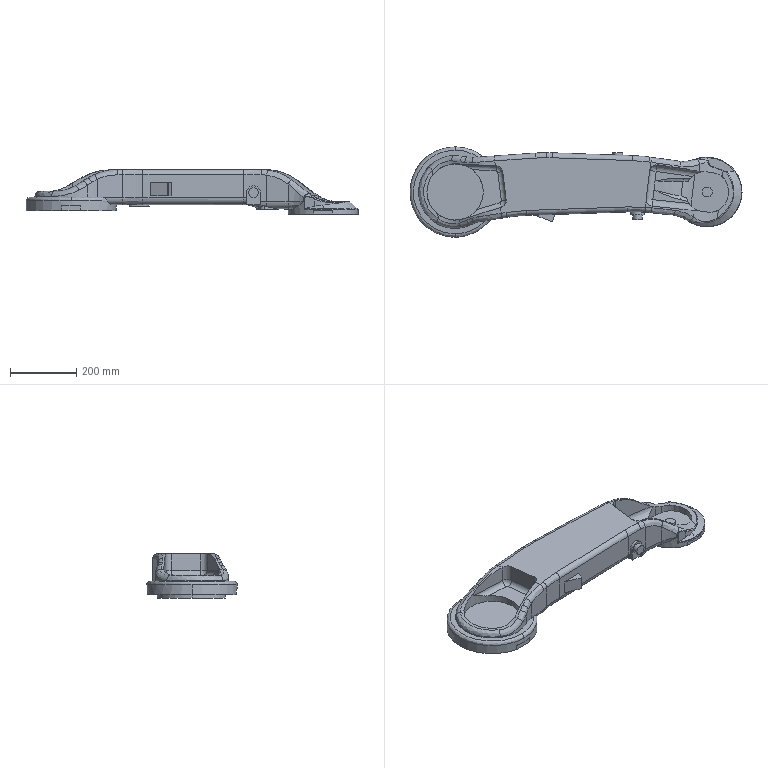Part | STEP file | Link2 | 1 solid | 224 faces | box 1001 x 272 x 134 mm | volume 13121493 mm3 | cylinder 88 | plane 67 | spline 57 | torus 6 | sphere 3 | cone 3 | commonest cylinder face diameters 30 x17 40 x15 24 x9 200 x6 6 x4 100 x4